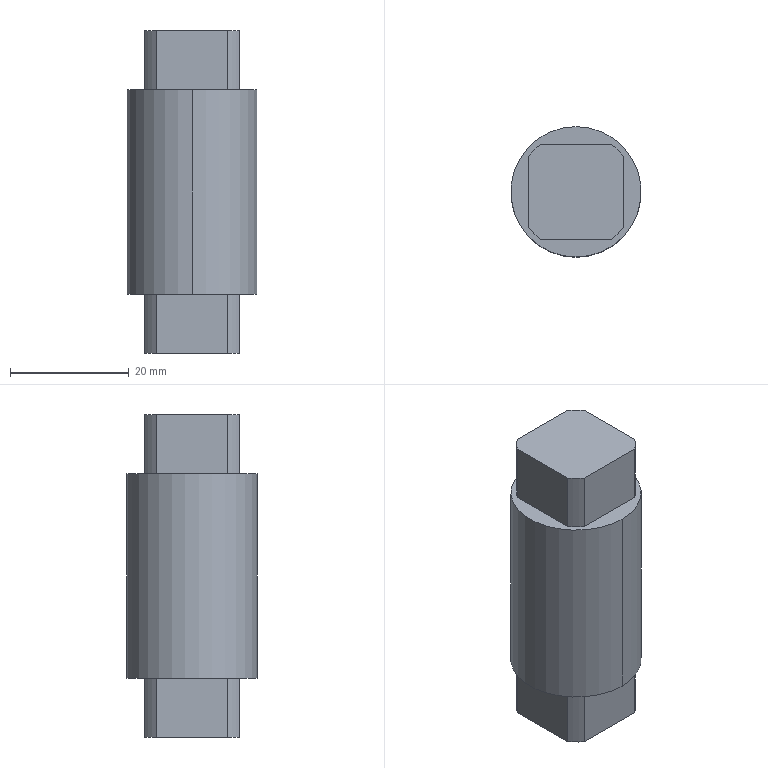Part | NX | features BREP 1 | 1 solid | 22 faces | box 22 x 22 x 54.5 mm | volume 18090 mm3 | plane 12 | cylinder 10 | commonest cylinder face diameters 20 x8 22 x2
STEP:
#1=CARTESIAN_POINT('',(6.,8.,27.25));
#2=VERTEX_POINT('',#1);
#3=CARTESIAN_POINT('',(6.,8.,17.25));
#4=VERTEX_POINT('',#3);
#5=CARTESIAN_POINT('',(6.,8.,27.25));
#6=DIRECTION('',(0.,0.,-1.));
#7=VECTOR('',#6,1000.);
#8=LINE('',#5,#7);
#9=EDGE_CURVE('',#2,#4,#8,.T.);
#10=ORIENTED_EDGE('',*,*,#9,.F.);
#11=CARTESIAN_POINT('',(8.,6.,27.25));
#12=VERTEX_POINT('',#11);
#13=CARTESIAN_POINT('',(0.,0.,27.25));
#14=DIRECTION('',(0.,0.,-1.));
#15=DIRECTION('',(0.6,0.8,0.));
#16=AXIS2_PLACEMENT_3D('',#13,#14,#15);
#17=CIRCLE('',#16,10.);
#18=EDGE_CURVE('',#2,#12,#17,.T.);
#19=ORIENTED_EDGE('',*,*,#18,.T.);
#20=CARTESIAN_POINT('',(8.,6.,17.25));
#21=VERTEX_POINT('',#20);
#22=CARTESIAN_POINT('',(8.,6.,27.25));
#23=DIRECTION('',(0.,0.,-1.));
#24=VECTOR('',#23,1000.);
#25=LINE('',#22,#24);
#26=EDGE_CURVE('',#12,#21,#25,.T.);
#27=ORIENTED_EDGE('',*,*,#26,.T.);
#28=CARTESIAN_POINT('',(0.,0.,17.25));
#29=DIRECTION('',(0.,0.,1.));
#30=DIRECTION('',(0.8,0.6,0.));
#31=AXIS2_PLACEMENT_3D('',#28,#29,#30);
#32=CIRCLE('',#31,10.);
#33=EDGE_CURVE('',#21,#4,#32,.T.);
#34=ORIENTED_EDGE('',*,*,#33,.T.);
#35=EDGE_LOOP('',(#10,#19,#27,#34));
#36=FACE_BOUND('',#35,.T.);
#37=CARTESIAN_POINT('',(0.,0.,27.25));
#38=DIRECTION('',(0.,0.,1.));
#39=DIRECTION('',(0.,1.,0.));
#40=AXIS2_PLACEMENT_3D('',#37,#38,#39);
#41=CYLINDRICAL_SURFACE('',#40,10.);
#42=ADVANCED_FACE('',(#36),#41,.T.);
#43=ORIENTED_EDGE('',*,*,#26,.F.);
#44=CARTESIAN_POINT('',(8.,-6.,27.25));
#45=VERTEX_POINT('',#44);
#46=CARTESIAN_POINT('',(8.,-6.,27.25));
#47=DIRECTION('',(0.,1.,0.));
#48=VECTOR('',#47,1000.);
#49=LINE('',#46,#48);
#50=EDGE_CURVE('',#45,#12,#49,.T.);
#51=ORIENTED_EDGE('',*,*,#50,.F.);
#52=CARTESIAN_POINT('',(8.,-6.,17.25));
#53=VERTEX_POINT('',#52);
#54=CARTESIAN_POINT('',(8.,-6.,27.25));
#55=DIRECTION('',(0.,0.,-1.));
#56=VECTOR('',#55,1000.);
#57=LINE('',#54,#56);
#58=EDGE_CURVE('',#45,#53,#57,.T.);
#59=ORIENTED_EDGE('',*,*,#58,.T.);
#60=CARTESIAN_POINT('',(8.,-6.,17.25));
#61=DIRECTION('',(0.,1.,0.));
#62=VECTOR('',#61,1000.);
#63=LINE('',#60,#62);
#64=EDGE_CURVE('',#53,#21,#63,.T.);
#65=ORIENTED_EDGE('',*,*,#64,.T.);
#66=EDGE_LOOP('',(#43,#51,#59,#65));
#67=FACE_BOUND('',#66,.T.);
#68=CARTESIAN_POINT('',(8.,-6.,27.25));
#69=DIRECTION('',(-1.,0.,0.));
#70=DIRECTION('',(0.,-1.,0.));
#71=AXIS2_PLACEMENT_3D('',#68,#69,#70);
#72=PLANE('',#71);
#73=ADVANCED_FACE('',(#67),#72,.F.);
#74=ORIENTED_EDGE('',*,*,#58,.F.);
#75=CARTESIAN_POINT('',(6.,-8.,27.25));
#76=VERTEX_POINT('',#75);
#77=CARTESIAN_POINT('',(0.,0.,27.25));
#78=DIRECTION('',(0.,0.,-1.));
#79=DIRECTION('',(0.8,-0.6,0.));
#80=AXIS2_PLACEMENT_3D('',#77,#78,#79);
#81=CIRCLE('',#80,10.);
#82=EDGE_CURVE('',#45,#76,#81,.T.);
#83=ORIENTED_EDGE('',*,*,#82,.T.);
#84=CARTESIAN_POINT('',(6.,-8.,17.25));
#85=VERTEX_POINT('',#84);
#86=CARTESIAN_POINT('',(6.,-8.,27.25));
#87=DIRECTION('',(0.,0.,-1.));
#88=VECTOR('',#87,1000.);
#89=LINE('',#86,#88);
#90=EDGE_CURVE('',#76,#85,#89,.T.);
#91=ORIENTED_EDGE('',*,*,#90,.T.);
#92=CARTESIAN_POINT('',(0.,0.,17.25));
#93=DIRECTION('',(0.,0.,1.));
#94=DIRECTION('',(0.6,-0.8,0.));
#95=AXIS2_PLACEMENT_3D('',#92,#93,#94);
#96=CIRCLE('',#95,10.);
#97=EDGE_CURVE('',#85,#53,#96,.T.);
#98=ORIENTED_EDGE('',*,*,#97,.T.);
#99=EDGE_LOOP('',(#74,#83,#91,#98));
#100=FACE_BOUND('',#99,.T.);
#101=CARTESIAN_POINT('',(0.,0.,27.25));
#102=DIRECTION('',(0.,0.,1.));
#103=DIRECTION('',(0.,1.,0.));
#104=AXIS2_PLACEMENT_3D('',#101,#102,#103);
#105=CYLINDRICAL_SURFACE('',#104,10.);
#106=ADVANCED_FACE('',(#100),#105,.T.);
#107=ORIENTED_EDGE('',*,*,#90,.F.);
#108=CARTESIAN_POINT('',(-6.,-8.,27.25));
#109=VERTEX_POINT('',#108);
#110=CARTESIAN_POINT('',(-6.,-8.,27.25));
#111=DIRECTION('',(1.,0.,0.));
#112=VECTOR('',#111,1000.);
#113=LINE('',#110,#112);
#114=EDGE_CURVE('',#109,#76,#113,.T.);
#115=ORIENTED_EDGE('',*,*,#114,.F.);
#116=CARTESIAN_POINT('',(-6.,-8.,17.25));
#117=VERTEX_POINT('',#116);
#118=CARTESIAN_POINT('',(-6.,-8.,27.25));
#119=DIRECTION('',(0.,0.,-1.));
#120=VECTOR('',#119,1000.);
#121=LINE('',#118,#120);
#122=EDGE_CURVE('',#109,#117,#121,.T.);
#123=ORIENTED_EDGE('',*,*,#122,.T.);
#124=CARTESIAN_POINT('',(-6.,-8.,17.25));
#125=DIRECTION('',(1.,0.,0.));
#126=VECTOR('',#125,1000.);
#127=LINE('',#124,#126);
#128=EDGE_CURVE('',#117,#85,#127,.T.);
#129=ORIENTED_EDGE('',*,*,#128,.T.);
#130=EDGE_LOOP('',(#107,#115,#123,#129));
#131=FACE_BOUND('',#130,.T.);
#132=CARTESIAN_POINT('',(-6.,-8.,27.25));
#133=DIRECTION('',(0.,1.,0.));
#134=DIRECTION('',(-1.,0.,0.));
#135=AXIS2_PLACEMENT_3D('',#132,#133,#134);
#136=PLANE('',#135);
#137=ADVANCED_FACE('',(#131),#136,.F.);
#138=ORIENTED_EDGE('',*,*,#122,.F.);
#139=CARTESIAN_POINT('',(-8.,-6.,27.25));
#140=VERTEX_POINT('',#139);
#141=CARTESIAN_POINT('',(0.,0.,27.25));
#142=DIRECTION('',(0.,0.,-1.));
#143=DIRECTION('',(-0.6,-0.8,0.));
#144=AXIS2_PLACEMENT_3D('',#141,#142,#143);
#145=CIRCLE('',#144,10.);
#146=EDGE_CURVE('',#109,#140,#145,.T.);
#147=ORIENTED_EDGE('',*,*,#146,.T.);
#148=CARTESIAN_POINT('',(-8.,-6.,17.25));
#149=VERTEX_POINT('',#148);
#150=CARTESIAN_POINT('',(-8.,-6.,27.25));
#151=DIRECTION('',(0.,0.,-1.));
#152=VECTOR('',#151,1000.);
#153=LINE('',#150,#152);
#154=EDGE_CURVE('',#140,#149,#153,.T.);
#155=ORIENTED_EDGE('',*,*,#154,.T.);
#156=CARTESIAN_POINT('',(0.,0.,17.25));
#157=DIRECTION('',(0.,0.,1.));
#158=DIRECTION('',(-0.8,-0.6,0.));
#159=AXIS2_PLACEMENT_3D('',#156,#157,#158);
#160=CIRCLE('',#159,10.);
#161=EDGE_CURVE('',#149,#117,#160,.T.);
#162=ORIENTED_EDGE('',*,*,#161,.T.);
#163=EDGE_LOOP('',(#138,#147,#155,#162));
#164=FACE_BOUND('',#163,.T.);
#165=CARTESIAN_POINT('',(0.,0.,27.25));
#166=DIRECTION('',(0.,0.,1.));
#167=DIRECTION('',(0.,1.,0.));
#168=AXIS2_PLACEMENT_3D('',#165,#166,#167);
#169=CYLINDRICAL_SURFACE('',#168,10.);
#170=ADVANCED_FACE('',(#164),#169,.T.);
#171=ORIENTED_EDGE('',*,*,#154,.F.);
#172=CARTESIAN_POINT('',(-8.,6.,27.25));
#173=VERTEX_POINT('',#172);
#174=CARTESIAN_POINT('',(-8.,6.,27.25));
#175=DIRECTION('',(0.,-1.,0.));
#176=VECTOR('',#175,1000.);
#177=LINE('',#174,#176);
#178=EDGE_CURVE('',#173,#140,#177,.T.);
#179=ORIENTED_EDGE('',*,*,#178,.F.);
#180=CARTESIAN_POINT('',(-8.,6.,17.25));
#181=VERTEX_POINT('',#180);
#182=CARTESIAN_POINT('',(-8.,6.,27.25));
#183=DIRECTION('',(0.,0.,-1.));
#184=VECTOR('',#183,1000.);
#185=LINE('',#182,#184);
#186=EDGE_CURVE('',#173,#181,#185,.T.);
#187=ORIENTED_EDGE('',*,*,#186,.T.);
#188=CARTESIAN_POINT('',(-8.,6.,17.25));
#189=DIRECTION('',(0.,-1.,0.));
#190=VECTOR('',#189,1000.);
#191=LINE('',#188,#190);
#192=EDGE_CURVE('',#181,#149,#191,.T.);
#193=ORIENTED_EDGE('',*,*,#192,.T.);
#194=EDGE_LOOP('',(#171,#179,#187,#193));
#195=FACE_BOUND('',#194,.T.);
#196=CARTESIAN_POINT('',(-8.,6.,27.25));
#197=DIRECTION('',(1.,0.,0.));
#198=DIRECTION('',(0.,1.,0.));
#199=AXIS2_PLACEMENT_3D('',#196,#197,#198);
#200=PLANE('',#199);
#201=ADVANCED_FACE('',(#195),#200,.F.);
#202=ORIENTED_EDGE('',*,*,#186,.F.);
#203=CARTESIAN_POINT('',(-6.,8.,27.25));
#204=VERTEX_POINT('',#203);
#205=CARTESIAN_POINT('',(0.,0.,27.25));
#206=DIRECTION('',(0.,0.,-1.));
#207=DIRECTION('',(-0.8,0.6,0.));
#208=AXIS2_PLACEMENT_3D('',#205,#206,#207);
#209=CIRCLE('',#208,10.);
#210=EDGE_CURVE('',#173,#204,#209,.T.);
#211=ORIENTED_EDGE('',*,*,#210,.T.);
#212=CARTESIAN_POINT('',(-6.,8.,17.25));
#213=VERTEX_POINT('',#212);
#214=CARTESIAN_POINT('',(-6.,8.,27.25));
#215=DIRECTION('',(0.,0.,-1.));
#216=VECTOR('',#215,1000.);
#217=LINE('',#214,#216);
#218=EDGE_CURVE('',#204,#213,#217,.T.);
#219=ORIENTED_EDGE('',*,*,#218,.T.);
#220=CARTESIAN_POINT('',(0.,0.,17.25));
#221=DIRECTION('',(0.,0.,1.));
#222=DIRECTION('',(-0.6,0.8,0.));
#223=AXIS2_PLACEMENT_3D('',#220,#221,#222);
#224=CIRCLE('',#223,10.);
#225=EDGE_CURVE('',#213,#181,#224,.T.);
#226=ORIENTED_EDGE('',*,*,#225,.T.);
#227=EDGE_LOOP('',(#202,#211,#219,#226));
#228=FACE_BOUND('',#227,.T.);
#229=CARTESIAN_POINT('',(0.,0.,27.25));
#230=DIRECTION('',(0.,0.,1.));
#231=DIRECTION('',(0.,1.,0.));
#232=AXIS2_PLACEMENT_3D('',#229,#230,#231);
#233=CYLINDRICAL_SURFACE('',#232,10.);
#234=ADVANCED_FACE('',(#228),#233,.T.);
#235=ORIENTED_EDGE('',*,*,#18,.F.);
#236=CARTESIAN_POINT('',(6.,8.,27.25));
#237=DIRECTION('',(-1.,0.,0.));
#238=VECTOR('',#237,1000.);
#239=LINE('',#236,#238);
#240=EDGE_CURVE('',#2,#204,#239,.T.);
#241=ORIENTED_EDGE('',*,*,#240,.T.);
#242=ORIENTED_EDGE('',*,*,#210,.F.);
#243=ORIENTED_EDGE('',*,*,#178,.T.);
#244=ORIENTED_EDGE('',*,*,#146,.F.);
#245=ORIENTED_EDGE('',*,*,#114,.T.);
#246=ORIENTED_EDGE('',*,*,#82,.F.);
#247=ORIENTED_EDGE('',*,*,#50,.T.);
#248=EDGE_LOOP('',(#235,#241,#242,#243,#244,#245,#246,#247));
#249=FACE_BOUND('',#248,.T.);
#250=CARTESIAN_POINT('',(0.,0.,27.25));
#251=DIRECTION('',(0.,0.,1.));
#252=DIRECTION('',(0.,1.,0.));
#253=AXIS2_PLACEMENT_3D('',#250,#251,#252);
#254=PLANE('',#253);
#255=ADVANCED_FACE('',(#249),#254,.T.);
#256=ORIENTED_EDGE('',*,*,#218,.F.);
#257=ORIENTED_EDGE('',*,*,#240,.F.);
#258=ORIENTED_EDGE('',*,*,#9,.T.);
#259=CARTESIAN_POINT('',(6.,8.,17.25));
#260=DIRECTION('',(-1.,0.,0.));
#261=VECTOR('',#260,1000.);
#262=LINE('',#259,#261);
#263=EDGE_CURVE('',#4,#213,#262,.T.);
#264=ORIENTED_EDGE('',*,*,#263,.T.);
#265=EDGE_LOOP('',(#256,#257,#258,#264));
#266=FACE_BOUND('',#265,.T.);
#267=CARTESIAN_POINT('',(6.,8.,27.25));
#268=DIRECTION('',(0.,-1.,0.));
#269=DIRECTION('',(1.,0.,0.));
#270=AXIS2_PLACEMENT_3D('',#267,#268,#269);
#271=PLANE('',#270);
#272=ADVANCED_FACE('',(#266),#271,.F.);
#273=CARTESIAN_POINT('',(0.,11.,17.25));
#274=VERTEX_POINT('',#273);
#275=CARTESIAN_POINT('',(0.,11.,-17.25));
#276=VERTEX_POINT('',#275);
#277=CARTESIAN_POINT('',(0.,11.,-17.25));
#278=DIRECTION('',(0.,0.,1.));
#279=VECTOR('',#278,1000.);
#280=LINE('',#277,#279);
#281=EDGE_CURVE('',#274,#276,#280,.F.);
#282=ORIENTED_EDGE('',*,*,#281,.F.);
#283=CARTESIAN_POINT('',(0.,-11.,17.25));
#284=VERTEX_POINT('',#283);
#285=CARTESIAN_POINT('',(0.,0.,17.25));
#286=DIRECTION('',(0.,0.,-1.));
#287=DIRECTION('',(0.,1.,0.));
#288=AXIS2_PLACEMENT_3D('',#285,#286,#287);
#289=CIRCLE('',#288,11.);
#290=EDGE_CURVE('',#274,#284,#289,.T.);
#291=ORIENTED_EDGE('',*,*,#290,.T.);
#292=CARTESIAN_POINT('',(0.,-11.,-17.25));
#293=VERTEX_POINT('',#292);
#294=CARTESIAN_POINT('',(0.,-11.,-17.25));
#295=DIRECTION('',(0.,0.,1.));
#296=VECTOR('',#295,1000.);
#297=LINE('',#294,#296);
#298=EDGE_CURVE('',#284,#293,#297,.F.);
#299=ORIENTED_EDGE('',*,*,#298,.T.);
#300=CARTESIAN_POINT('',(0.,0.,-17.25));
#301=DIRECTION('',(0.,0.,-1.));
#302=DIRECTION('',(0.,1.,0.));
#303=AXIS2_PLACEMENT_3D('',#300,#301,#302);
#304=CIRCLE('',#303,11.);
#305=EDGE_CURVE('',#276,#293,#304,.T.);
#306=ORIENTED_EDGE('',*,*,#305,.F.);
#307=EDGE_LOOP('',(#282,#291,#299,#306));
#308=FACE_BOUND('',#307,.T.);
#309=CARTESIAN_POINT('',(0.,0.,0.));
#310=DIRECTION('',(0.,0.,1.));
#311=DIRECTION('',(0.,1.,0.));
#312=AXIS2_PLACEMENT_3D('',#309,#310,#311);
#313=CYLINDRICAL_SURFACE('',#312,11.);
#314=ADVANCED_FACE('',(#308),#313,.T.);
#315=ORIENTED_EDGE('',*,*,#225,.F.);
#316=ORIENTED_EDGE('',*,*,#263,.F.);
#317=ORIENTED_EDGE('',*,*,#33,.F.);
#318=ORIENTED_EDGE('',*,*,#64,.F.);
#319=ORIENTED_EDGE('',*,*,#97,.F.);
#320=ORIENTED_EDGE('',*,*,#128,.F.);
#321=ORIENTED_EDGE('',*,*,#161,.F.);
#322=ORIENTED_EDGE('',*,*,#192,.F.);
#323=EDGE_LOOP('',(#315,#316,#317,#318,#319,#320,#321,#322));
#324=FACE_BOUND('',#323,.T.);
#325=ORIENTED_EDGE('',*,*,#290,.F.);
#326=CARTESIAN_POINT('',(0.,0.,17.25));
#327=DIRECTION('',(0.,0.,-1.));
#328=DIRECTION('',(0.,-1.,0.));
#329=AXIS2_PLACEMENT_3D('',#326,#327,#328);
#330=CIRCLE('',#329,11.);
#331=EDGE_CURVE('',#284,#274,#330,.T.);
#332=ORIENTED_EDGE('',*,*,#331,.F.);
#333=EDGE_LOOP('',(#325,#332));
#334=FACE_BOUND('',#333,.T.);
#335=CARTESIAN_POINT('',(0.,0.,17.25));
#336=DIRECTION('',(0.,0.,1.));
#337=DIRECTION('',(0.,1.,0.));
#338=AXIS2_PLACEMENT_3D('',#335,#336,#337);
#339=PLANE('',#338);
#340=ADVANCED_FACE('',(#324,#334),#339,.T.);
#341=ORIENTED_EDGE('',*,*,#298,.F.);
#342=ORIENTED_EDGE('',*,*,#331,.T.);
#343=ORIENTED_EDGE('',*,*,#281,.T.);
#344=CARTESIAN_POINT('',(0.,0.,-17.25));
#345=DIRECTION('',(0.,0.,-1.));
#346=DIRECTION('',(0.,-1.,0.));
#347=AXIS2_PLACEMENT_3D('',#344,#345,#346);
#348=CIRCLE('',#347,11.);
#349=EDGE_CURVE('',#293,#276,#348,.T.);
#350=ORIENTED_EDGE('',*,*,#349,.F.);
#351=EDGE_LOOP('',(#341,#342,#343,#350));
#352=FACE_BOUND('',#351,.T.);
#353=CARTESIAN_POINT('',(0.,0.,0.));
#354=DIRECTION('',(0.,0.,1.));
#355=DIRECTION('',(0.,1.,0.));
#356=AXIS2_PLACEMENT_3D('',#353,#354,#355);
#357=CYLINDRICAL_SURFACE('',#356,11.);
#358=ADVANCED_FACE('',(#352),#357,.T.);
#359=CARTESIAN_POINT('',(6.,8.,-17.25));
#360=VERTEX_POINT('',#359);
#361=CARTESIAN_POINT('',(8.,6.,-17.25));
#362=VERTEX_POINT('',#361);
#363=CARTESIAN_POINT('',(0.,0.,-17.25));
#364=DIRECTION('',(0.,0.,-1.));
#365=DIRECTION('',(0.6,0.8,0.));
#366=AXIS2_PLACEMENT_3D('',#363,#364,#365);
#367=CIRCLE('',#366,10.);
#368=EDGE_CURVE('',#360,#362,#367,.T.);
#369=ORIENTED_EDGE('',*,*,#368,.F.);
#370=CARTESIAN_POINT('',(-6.,8.,-17.25));
#371=VERTEX_POINT('',#370);
#372=CARTESIAN_POINT('',(-6.,8.,-17.25));
#373=DIRECTION('',(1.,0.,0.));
#374=VECTOR('',#373,1000.);
#375=LINE('',#372,#374);
#376=EDGE_CURVE('',#371,#360,#375,.T.);
#377=ORIENTED_EDGE('',*,*,#376,.F.);
#378=CARTESIAN_POINT('',(-8.,6.,-17.25));
#379=VERTEX_POINT('',#378);
#380=CARTESIAN_POINT('',(0.,0.,-17.25));
#381=DIRECTION('',(0.,0.,-1.));
#382=DIRECTION('',(-0.8,0.6,0.));
#383=AXIS2_PLACEMENT_3D('',#380,#381,#382);
#384=CIRCLE('',#383,10.);
#385=EDGE_CURVE('',#379,#371,#384,.T.);
#386=ORIENTED_EDGE('',*,*,#385,.F.);
#387=CARTESIAN_POINT('',(-8.,-6.,-17.25));
#388=VERTEX_POINT('',#387);
#389=CARTESIAN_POINT('',(-8.,-6.,-17.25));
#390=DIRECTION('',(0.,1.,0.));
#391=VECTOR('',#390,1000.);
#392=LINE('',#389,#391);
#393=EDGE_CURVE('',#388,#379,#392,.T.);
#394=ORIENTED_EDGE('',*,*,#393,.F.);
#395=CARTESIAN_POINT('',(-6.,-8.,-17.25));
#396=VERTEX_POINT('',#395);
#397=CARTESIAN_POINT('',(0.,0.,-17.25));
#398=DIRECTION('',(0.,0.,-1.));
#399=DIRECTION('',(-0.6,-0.8,0.));
#400=AXIS2_PLACEMENT_3D('',#397,#398,#399);
#401=CIRCLE('',#400,10.);
#402=EDGE_CURVE('',#396,#388,#401,.T.);
#403=ORIENTED_EDGE('',*,*,#402,.F.);
#404=CARTESIAN_POINT('',(6.,-8.,-17.25));
#405=VERTEX_POINT('',#404);
#406=CARTESIAN_POINT('',(6.,-8.,-17.25));
#407=DIRECTION('',(-1.,0.,0.));
#408=VECTOR('',#407,1000.);
#409=LINE('',#406,#408);
#410=EDGE_CURVE('',#405,#396,#409,.T.);
#411=ORIENTED_EDGE('',*,*,#410,.F.);
#412=CARTESIAN_POINT('',(8.,-6.,-17.25));
#413=VERTEX_POINT('',#412);
#414=CARTESIAN_POINT('',(0.,0.,-17.25));
#415=DIRECTION('',(0.,0.,-1.));
#416=DIRECTION('',(0.8,-0.6,0.));
#417=AXIS2_PLACEMENT_3D('',#414,#415,#416);
#418=CIRCLE('',#417,10.);
#419=EDGE_CURVE('',#413,#405,#418,.T.);
#420=ORIENTED_EDGE('',*,*,#419,.F.);
#421=CARTESIAN_POINT('',(8.,6.,-17.25));
#422=DIRECTION('',(0.,-1.,0.));
#423=VECTOR('',#422,1000.);
#424=LINE('',#421,#423);
#425=EDGE_CURVE('',#362,#413,#424,.T.);
#426=ORIENTED_EDGE('',*,*,#425,.F.);
#427=EDGE_LOOP('',(#369,#377,#386,#394,#403,#411,#420,#426));
#428=FACE_BOUND('',#427,.T.);
#429=ORIENTED_EDGE('',*,*,#305,.T.);
#430=ORIENTED_EDGE('',*,*,#349,.T.);
#431=EDGE_LOOP('',(#429,#430));
#432=FACE_BOUND('',#431,.T.);
#433=CARTESIAN_POINT('',(0.,0.,-17.25));
#434=DIRECTION('',(0.,0.,-1.));
#435=DIRECTION('',(0.,1.,0.));
#436=AXIS2_PLACEMENT_3D('',#433,#434,#435);
#437=PLANE('',#436);
#438=ADVANCED_FACE('',(#428,#432),#437,.T.);
#439=CARTESIAN_POINT('',(8.,6.,-27.25));
#440=VERTEX_POINT('',#439);
#441=CARTESIAN_POINT('',(8.,6.,-27.25));
#442=DIRECTION('',(0.,0.,1.));
#443=VECTOR('',#442,1000.);
#444=LINE('',#441,#443);
#445=EDGE_CURVE('',#440,#362,#444,.T.);
#446=ORIENTED_EDGE('',*,*,#445,.F.);
#447=CARTESIAN_POINT('',(6.,8.,-27.25));
#448=VERTEX_POINT('',#447);
#449=CARTESIAN_POINT('',(0.,0.,-27.25));
#450=DIRECTION('',(0.,0.,1.));
#451=DIRECTION('',(0.8,0.6,0.));
#452=AXIS2_PLACEMENT_3D('',#449,#450,#451);
#453=CIRCLE('',#452,10.);
#454=EDGE_CURVE('',#440,#448,#453,.T.);
#455=ORIENTED_EDGE('',*,*,#454,.T.);
#456=CARTESIAN_POINT('',(6.,8.,-27.25));
#457=DIRECTION('',(0.,0.,1.));
#458=VECTOR('',#457,1000.);
#459=LINE('',#456,#458);
#460=EDGE_CURVE('',#448,#360,#459,.T.);
#461=ORIENTED_EDGE('',*,*,#460,.T.);
#462=ORIENTED_EDGE('',*,*,#368,.T.);
#463=EDGE_LOOP('',(#446,#455,#461,#462));
#464=FACE_BOUND('',#463,.T.);
#465=CARTESIAN_POINT('',(0.,0.,-27.25));
#466=DIRECTION('',(0.,0.,-1.));
#467=DIRECTION('',(0.,1.,0.));
#468=AXIS2_PLACEMENT_3D('',#465,#466,#467);
#469=CYLINDRICAL_SURFACE('',#468,10.);
#470=ADVANCED_FACE('',(#464),#469,.T.);
#471=CARTESIAN_POINT('',(8.,-6.,-27.25));
#472=VERTEX_POINT('',#471);
#473=CARTESIAN_POINT('',(8.,-6.,-27.25));
#474=DIRECTION('',(0.,0.,1.));
#475=VECTOR('',#474,1000.);
#476=LINE('',#473,#475);
#477=EDGE_CURVE('',#472,#413,#476,.T.);
#478=ORIENTED_EDGE('',*,*,#477,.F.);
#479=CARTESIAN_POINT('',(8.,6.,-27.25));
#480=DIRECTION('',(0.,-1.,0.));
#481=VECTOR('',#480,1000.);
#482=LINE('',#479,#481);
#483=EDGE_CURVE('',#440,#472,#482,.T.);
#484=ORIENTED_EDGE('',*,*,#483,.F.);
#485=ORIENTED_EDGE('',*,*,#445,.T.);
#486=ORIENTED_EDGE('',*,*,#425,.T.);
#487=EDGE_LOOP('',(#478,#484,#485,#486));
#488=FACE_BOUND('',#487,.T.);
#489=CARTESIAN_POINT('',(8.,6.,-27.25));
#490=DIRECTION('',(-1.,0.,0.));
#491=DIRECTION('',(0.,1.,0.));
#492=AXIS2_PLACEMENT_3D('',#489,#490,#491);
#493=PLANE('',#492);
#494=ADVANCED_FACE('',(#488),#493,.F.);
#495=CARTESIAN_POINT('',(6.,-8.,-27.25));
#496=VERTEX_POINT('',#495);
#497=CARTESIAN_POINT('',(6.,-8.,-27.25));
#498=DIRECTION('',(0.,0.,1.));
#499=VECTOR('',#498,1000.);
#500=LINE('',#497,#499);
#501=EDGE_CURVE('',#496,#405,#500,.T.);
#502=ORIENTED_EDGE('',*,*,#501,.F.);
#503=CARTESIAN_POINT('',(0.,0.,-27.25));
#504=DIRECTION('',(0.,0.,1.));
#505=DIRECTION('',(0.6,-0.8,0.));
#506=AXIS2_PLACEMENT_3D('',#503,#504,#505);
#507=CIRCLE('',#506,10.);
#508=EDGE_CURVE('',#496,#472,#507,.T.);
#509=ORIENTED_EDGE('',*,*,#508,.T.);
#510=ORIENTED_EDGE('',*,*,#477,.T.);
#511=ORIENTED_EDGE('',*,*,#419,.T.);
#512=EDGE_LOOP('',(#502,#509,#510,#511));
#513=FACE_BOUND('',#512,.T.);
#514=CARTESIAN_POINT('',(0.,0.,-27.25));
#515=DIRECTION('',(0.,0.,-1.));
#516=DIRECTION('',(0.,1.,0.));
#517=AXIS2_PLACEMENT_3D('',#514,#515,#516);
#518=CYLINDRICAL_SURFACE('',#517,10.);
#519=ADVANCED_FACE('',(#513),#518,.T.);
#520=CARTESIAN_POINT('',(-6.,-8.,-27.25));
#521=VERTEX_POINT('',#520);
#522=CARTESIAN_POINT('',(-6.,-8.,-27.25));
#523=DIRECTION('',(0.,0.,1.));
#524=VECTOR('',#523,1000.);
#525=LINE('',#522,#524);
#526=EDGE_CURVE('',#521,#396,#525,.T.);
#527=ORIENTED_EDGE('',*,*,#526,.F.);
#528=CARTESIAN_POINT('',(6.,-8.,-27.25));
#529=DIRECTION('',(-1.,0.,0.));
#530=VECTOR('',#529,1000.);
#531=LINE('',#528,#530);
#532=EDGE_CURVE('',#496,#521,#531,.T.);
#533=ORIENTED_EDGE('',*,*,#532,.F.);
#534=ORIENTED_EDGE('',*,*,#501,.T.);
#535=ORIENTED_EDGE('',*,*,#410,.T.);
#536=EDGE_LOOP('',(#527,#533,#534,#535));
#537=FACE_BOUND('',#536,.T.);
#538=CARTESIAN_POINT('',(6.,-8.,-27.25));
#539=DIRECTION('',(0.,1.,0.));
#540=DIRECTION('',(1.,0.,0.));
#541=AXIS2_PLACEMENT_3D('',#538,#539,#540);
#542=PLANE('',#541);
#543=ADVANCED_FACE('',(#537),#542,.F.);
#544=CARTESIAN_POINT('',(-8.,-6.,-27.25));
#545=VERTEX_POINT('',#544);
#546=CARTESIAN_POINT('',(-8.,-6.,-27.25));
#547=DIRECTION('',(0.,0.,1.));
#548=VECTOR('',#547,1000.);
#549=LINE('',#546,#548);
#550=EDGE_CURVE('',#545,#388,#549,.T.);
#551=ORIENTED_EDGE('',*,*,#550,.F.);
#552=CARTESIAN_POINT('',(0.,0.,-27.25));
#553=DIRECTION('',(0.,0.,1.));
#554=DIRECTION('',(-0.8,-0.6,0.));
#555=AXIS2_PLACEMENT_3D('',#552,#553,#554);
#556=CIRCLE('',#555,10.);
#557=EDGE_CURVE('',#545,#521,#556,.T.);
#558=ORIENTED_EDGE('',*,*,#557,.T.);
#559=ORIENTED_EDGE('',*,*,#526,.T.);
#560=ORIENTED_EDGE('',*,*,#402,.T.);
#561=EDGE_LOOP('',(#551,#558,#559,#560));
#562=FACE_BOUND('',#561,.T.);
#563=CARTESIAN_POINT('',(0.,0.,-27.25));
#564=DIRECTION('',(0.,0.,-1.));
#565=DIRECTION('',(0.,1.,0.));
#566=AXIS2_PLACEMENT_3D('',#563,#564,#565);
#567=CYLINDRICAL_SURFACE('',#566,10.);
#568=ADVANCED_FACE('',(#562),#567,.T.);
#569=CARTESIAN_POINT('',(-8.,6.,-27.25));
#570=VERTEX_POINT('',#569);
#571=CARTESIAN_POINT('',(-8.,6.,-27.25));
#572=DIRECTION('',(0.,0.,1.));
#573=VECTOR('',#572,1000.);
#574=LINE('',#571,#573);
#575=EDGE_CURVE('',#570,#379,#574,.T.);
#576=ORIENTED_EDGE('',*,*,#575,.F.);
#577=CARTESIAN_POINT('',(-8.,-6.,-27.25));
#578=DIRECTION('',(0.,1.,0.));
#579=VECTOR('',#578,1000.);
#580=LINE('',#577,#579);
#581=EDGE_CURVE('',#545,#570,#580,.T.);
#582=ORIENTED_EDGE('',*,*,#581,.F.);
#583=ORIENTED_EDGE('',*,*,#550,.T.);
#584=ORIENTED_EDGE('',*,*,#393,.T.);
#585=EDGE_LOOP('',(#576,#582,#583,#584));
#586=FACE_BOUND('',#585,.T.);
#587=CARTESIAN_POINT('',(-8.,-6.,-27.25));
#588=DIRECTION('',(1.,0.,0.));
#589=DIRECTION('',(0.,-1.,0.));
#590=AXIS2_PLACEMENT_3D('',#587,#588,#589);
#591=PLANE('',#590);
#592=ADVANCED_FACE('',(#586),#591,.F.);
#593=CARTESIAN_POINT('',(-6.,8.,-27.25));
#594=VERTEX_POINT('',#593);
#595=CARTESIAN_POINT('',(-6.,8.,-27.25));
#596=DIRECTION('',(0.,0.,1.));
#597=VECTOR('',#596,1000.);
#598=LINE('',#595,#597);
#599=EDGE_CURVE('',#594,#371,#598,.T.);
#600=ORIENTED_EDGE('',*,*,#599,.F.);
#601=CARTESIAN_POINT('',(0.,0.,-27.25));
#602=DIRECTION('',(0.,0.,1.));
#603=DIRECTION('',(-0.6,0.8,0.));
#604=AXIS2_PLACEMENT_3D('',#601,#602,#603);
#605=CIRCLE('',#604,10.);
#606=EDGE_CURVE('',#594,#570,#605,.T.);
#607=ORIENTED_EDGE('',*,*,#606,.T.);
#608=ORIENTED_EDGE('',*,*,#575,.T.);
#609=ORIENTED_EDGE('',*,*,#385,.T.);
#610=EDGE_LOOP('',(#600,#607,#608,#609));
#611=FACE_BOUND('',#610,.T.);
#612=CARTESIAN_POINT('',(0.,0.,-27.25));
#613=DIRECTION('',(0.,0.,-1.));
#614=DIRECTION('',(0.,1.,0.));
#615=AXIS2_PLACEMENT_3D('',#612,#613,#614);
#616=CYLINDRICAL_SURFACE('',#615,10.);
#617=ADVANCED_FACE('',(#611),#616,.T.);
#618=ORIENTED_EDGE('',*,*,#460,.F.);
#619=CARTESIAN_POINT('',(-6.,8.,-27.25));
#620=DIRECTION('',(1.,0.,0.));
#621=VECTOR('',#620,1000.);
#622=LINE('',#619,#621);
#623=EDGE_CURVE('',#594,#448,#622,.T.);
#624=ORIENTED_EDGE('',*,*,#623,.F.);
#625=ORIENTED_EDGE('',*,*,#599,.T.);
#626=ORIENTED_EDGE('',*,*,#376,.T.);
#627=EDGE_LOOP('',(#618,#624,#625,#626));
#628=FACE_BOUND('',#627,.T.);
#629=CARTESIAN_POINT('',(-6.,8.,-27.25));
#630=DIRECTION('',(0.,-1.,0.));
#631=DIRECTION('',(-1.,0.,0.));
#632=AXIS2_PLACEMENT_3D('',#629,#630,#631);
#633=PLANE('',#632);
#634=ADVANCED_FACE('',(#628),#633,.F.);
#635=ORIENTED_EDGE('',*,*,#606,.F.);
#636=ORIENTED_EDGE('',*,*,#623,.T.);
#637=ORIENTED_EDGE('',*,*,#454,.F.);
#638=ORIENTED_EDGE('',*,*,#483,.T.);
#639=ORIENTED_EDGE('',*,*,#508,.F.);
#640=ORIENTED_EDGE('',*,*,#532,.T.);
#641=ORIENTED_EDGE('',*,*,#557,.F.);
#642=ORIENTED_EDGE('',*,*,#581,.T.);
#643=EDGE_LOOP('',(#635,#636,#637,#638,#639,#640,#641,#642));
#644=FACE_BOUND('',#643,.T.);
#645=CARTESIAN_POINT('',(0.,0.,-27.25));
#646=DIRECTION('',(0.,0.,1.));
#647=DIRECTION('',(0.,1.,0.));
#648=AXIS2_PLACEMENT_3D('',#645,#646,#647);
#649=PLANE('',#648);
#650=ADVANCED_FACE('',(#644),#649,.F.);
#651=CLOSED_SHELL('',(#42,#73,#106,#137,#170,#201,#234,#255,#272,#314,#340,#358,#438,#470,#494,#519,#543,#568,#592,#617,#634,#650));
#652=MANIFOLD_SOLID_BREP('',#651);
#653=(LENGTH_UNIT()NAMED_UNIT(*)SI_UNIT(.MILLI.,.METRE.));
#654=UNCERTAINTY_MEASURE_WITH_UNIT(LENGTH_MEASURE(0.00001),#653,'','');
#655=(NAMED_UNIT(*)PLANE_ANGLE_UNIT()SI_UNIT($,.RADIAN.));
#656=(NAMED_UNIT(*)SI_UNIT($,.STERADIAN.)SOLID_ANGLE_UNIT());
#657=(GEOMETRIC_REPRESENTATION_CONTEXT(3)GLOBAL_UNCERTAINTY_ASSIGNED_CONTEXT((#654))GLOBAL_UNIT_ASSIGNED_CONTEXT((#653,#655,#656))REPRESENTATION_CONTEXT('',''));
#658=ADVANCED_BREP_SHAPE_REPRESENTATION('',(#652),#657);